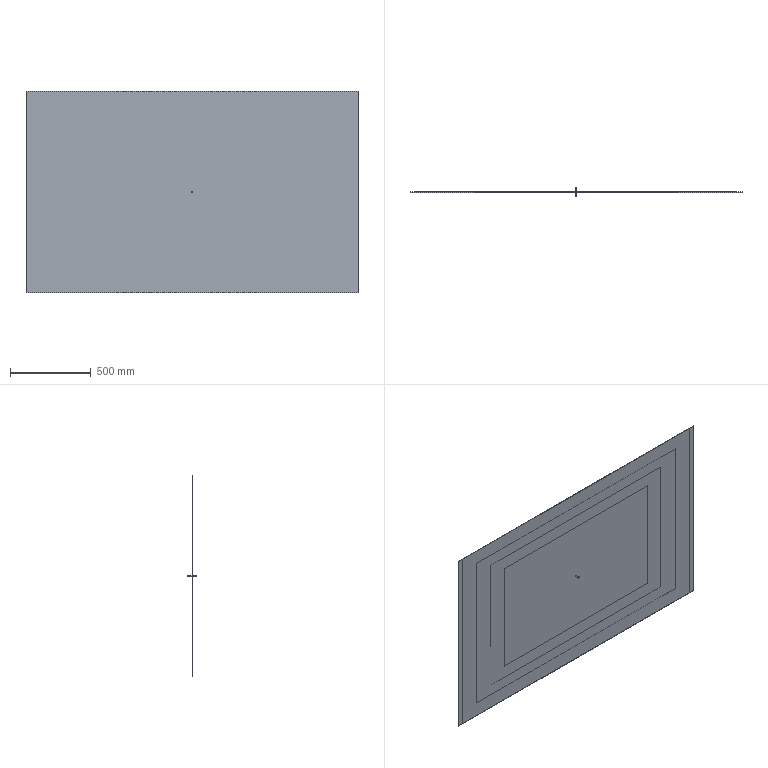Part | SolidWorks | features ICE 5, Extrusion 1 | 5 solids | 36 faces | box 2060 x 50 x 1250 mm | volume 5816564 mm3 | plane 32 | cylinder 4 | commonest cylinder face diameters 10 x4
STEP:
#1=CARTESIAN_POINT('',(1030.,-1.,625.));
#2=VERTEX_POINT('',#1);
#3=CARTESIAN_POINT('',(1030.,-1.,-625.));
#4=VERTEX_POINT('',#3);
#5=CARTESIAN_POINT('',(1030.,-1.,625.));
#6=DIRECTION('',(0.,0.,-1.));
#7=VECTOR('',#6,1000.);
#8=LINE('',#5,#7);
#9=EDGE_CURVE('',#2,#4,#8,.T.);
#10=ORIENTED_EDGE('',*,*,#9,.T.);
#11=CARTESIAN_POINT('',(1030.,1.,-625.));
#12=VERTEX_POINT('',#11);
#13=CARTESIAN_POINT('',(1030.,1.,-625.));
#14=DIRECTION('',(0.,-1.,0.));
#15=VECTOR('',#14,1000.);
#16=LINE('',#13,#15);
#17=EDGE_CURVE('',#12,#4,#16,.T.);
#18=ORIENTED_EDGE('',*,*,#17,.F.);
#19=CARTESIAN_POINT('',(1030.,1.,625.));
#20=VERTEX_POINT('',#19);
#21=CARTESIAN_POINT('',(1030.,1.,625.));
#22=DIRECTION('',(0.,0.,-1.));
#23=VECTOR('',#22,1000.);
#24=LINE('',#21,#23);
#25=EDGE_CURVE('',#20,#12,#24,.T.);
#26=ORIENTED_EDGE('',*,*,#25,.F.);
#27=CARTESIAN_POINT('',(1030.,1.,625.));
#28=DIRECTION('',(0.,-1.,0.));
#29=VECTOR('',#28,1000.);
#30=LINE('',#27,#29);
#31=EDGE_CURVE('',#20,#2,#30,.T.);
#32=ORIENTED_EDGE('',*,*,#31,.T.);
#33=EDGE_LOOP('',(#10,#18,#26,#32));
#34=FACE_OUTER_BOUND('',#33,.T.);
#35=CARTESIAN_POINT('',(1030.,1.,625.));
#36=DIRECTION('',(-1.,0.,0.));
#37=DIRECTION('',(0.,0.,1.));
#38=AXIS2_PLACEMENT_3D('',#35,#36,#37);
#39=PLANE('',#38);
#40=ADVANCED_FACE('',(#34),#39,.F.);
#41=CARTESIAN_POINT('',(-1030.,-1.,-625.));
#42=VERTEX_POINT('',#41);
#43=CARTESIAN_POINT('',(-1030.,-1.,-625.));
#44=DIRECTION('',(-1.,0.,0.));
#45=VECTOR('',#44,1000.);
#46=LINE('',#43,#45);
#47=EDGE_CURVE('',#4,#42,#46,.T.);
#48=ORIENTED_EDGE('',*,*,#47,.T.);
#49=CARTESIAN_POINT('',(-1030.,1.,-625.));
#50=VERTEX_POINT('',#49);
#51=CARTESIAN_POINT('',(-1030.,1.,-625.));
#52=DIRECTION('',(0.,-1.,0.));
#53=VECTOR('',#52,1000.);
#54=LINE('',#51,#53);
#55=EDGE_CURVE('',#50,#42,#54,.T.);
#56=ORIENTED_EDGE('',*,*,#55,.F.);
#57=CARTESIAN_POINT('',(-1030.,1.,-625.));
#58=DIRECTION('',(-1.,0.,0.));
#59=VECTOR('',#58,1000.);
#60=LINE('',#57,#59);
#61=EDGE_CURVE('',#12,#50,#60,.T.);
#62=ORIENTED_EDGE('',*,*,#61,.F.);
#63=ORIENTED_EDGE('',*,*,#17,.T.);
#64=EDGE_LOOP('',(#48,#56,#62,#63));
#65=FACE_OUTER_BOUND('',#64,.T.);
#66=CARTESIAN_POINT('',(-1030.,1.,-625.));
#67=DIRECTION('',(0.,0.,1.));
#68=DIRECTION('',(1.,0.,0.));
#69=AXIS2_PLACEMENT_3D('',#66,#67,#68);
#70=PLANE('',#69);
#71=ADVANCED_FACE('',(#65),#70,.F.);
#72=CARTESIAN_POINT('',(-1030.,-1.,625.));
#73=VERTEX_POINT('',#72);
#74=CARTESIAN_POINT('',(-1030.,-1.,625.));
#75=DIRECTION('',(0.,0.,1.));
#76=VECTOR('',#75,1000.);
#77=LINE('',#74,#76);
#78=EDGE_CURVE('',#42,#73,#77,.T.);
#79=ORIENTED_EDGE('',*,*,#78,.T.);
#80=CARTESIAN_POINT('',(-1030.,1.,625.));
#81=VERTEX_POINT('',#80);
#82=CARTESIAN_POINT('',(-1030.,1.,625.));
#83=DIRECTION('',(0.,-1.,0.));
#84=VECTOR('',#83,1000.);
#85=LINE('',#82,#84);
#86=EDGE_CURVE('',#81,#73,#85,.T.);
#87=ORIENTED_EDGE('',*,*,#86,.F.);
#88=CARTESIAN_POINT('',(-1030.,1.,625.));
#89=DIRECTION('',(0.,0.,1.));
#90=VECTOR('',#89,1000.);
#91=LINE('',#88,#90);
#92=EDGE_CURVE('',#50,#81,#91,.T.);
#93=ORIENTED_EDGE('',*,*,#92,.F.);
#94=ORIENTED_EDGE('',*,*,#55,.T.);
#95=EDGE_LOOP('',(#79,#87,#93,#94));
#96=FACE_OUTER_BOUND('',#95,.T.);
#97=CARTESIAN_POINT('',(-1030.,1.,625.));
#98=DIRECTION('',(1.,0.,0.));
#99=DIRECTION('',(0.,0.,-1.));
#100=AXIS2_PLACEMENT_3D('',#97,#98,#99);
#101=PLANE('',#100);
#102=ADVANCED_FACE('',(#96),#101,.F.);
#103=CARTESIAN_POINT('',(-1030.,-1.,625.));
#104=DIRECTION('',(1.,0.,0.));
#105=VECTOR('',#104,1000.);
#106=LINE('',#103,#105);
#107=EDGE_CURVE('',#73,#2,#106,.T.);
#108=ORIENTED_EDGE('',*,*,#107,.T.);
#109=ORIENTED_EDGE('',*,*,#31,.F.);
#110=CARTESIAN_POINT('',(-1030.,1.,625.));
#111=DIRECTION('',(1.,0.,0.));
#112=VECTOR('',#111,1000.);
#113=LINE('',#110,#112);
#114=EDGE_CURVE('',#81,#20,#113,.T.);
#115=ORIENTED_EDGE('',*,*,#114,.F.);
#116=ORIENTED_EDGE('',*,*,#86,.T.);
#117=EDGE_LOOP('',(#108,#109,#115,#116));
#118=FACE_OUTER_BOUND('',#117,.T.);
#119=CARTESIAN_POINT('',(-1030.,1.,625.));
#120=DIRECTION('',(0.,0.,-1.));
#121=DIRECTION('',(-1.,0.,0.));
#122=AXIS2_PLACEMENT_3D('',#119,#120,#121);
#123=PLANE('',#122);
#124=ADVANCED_FACE('',(#118),#123,.F.);
#125=ORIENTED_EDGE('',*,*,#25,.T.);
#126=ORIENTED_EDGE('',*,*,#61,.T.);
#127=ORIENTED_EDGE('',*,*,#92,.T.);
#128=ORIENTED_EDGE('',*,*,#114,.T.);
#129=EDGE_LOOP('',(#125,#126,#127,#128));
#130=FACE_OUTER_BOUND('',#129,.T.);
#131=CARTESIAN_POINT('',(0.,1.,0.));
#132=DIRECTION('',(0.,-1.,0.));
#133=DIRECTION('',(0.,0.,-1.));
#134=AXIS2_PLACEMENT_3D('',#131,#132,#133);
#135=PLANE('',#134);
#136=ADVANCED_FACE('',(#130),#135,.F.);
#137=ORIENTED_EDGE('',*,*,#9,.F.);
#138=ORIENTED_EDGE('',*,*,#107,.F.);
#139=ORIENTED_EDGE('',*,*,#78,.F.);
#140=ORIENTED_EDGE('',*,*,#47,.F.);
#141=EDGE_LOOP('',(#137,#138,#139,#140));
#142=FACE_OUTER_BOUND('',#141,.T.);
#143=CARTESIAN_POINT('',(0.,-1.,0.));
#144=DIRECTION('',(0.,-1.,0.));
#145=DIRECTION('',(0.,0.,-1.));
#146=AXIS2_PLACEMENT_3D('',#143,#144,#145);
#147=PLANE('',#146);
#148=ADVANCED_FACE('',(#142),#147,.T.);
#149=CLOSED_SHELL('',(#40,#71,#102,#124,#136,#148));
#150=MANIFOLD_SOLID_BREP('',#149);
#151=CARTESIAN_POINT('',(997.5,1.,625.));
#152=VERTEX_POINT('',#151);
#153=CARTESIAN_POINT('',(997.5,1.,-625.));
#154=VERTEX_POINT('',#153);
#155=CARTESIAN_POINT('',(997.5,1.,625.));
#156=DIRECTION('',(0.,0.,-1.));
#157=VECTOR('',#156,1000.);
#158=LINE('',#155,#157);
#159=EDGE_CURVE('',#152,#154,#158,.T.);
#160=ORIENTED_EDGE('',*,*,#159,.T.);
#161=CARTESIAN_POINT('',(997.5,1.1,-625.));
#162=VERTEX_POINT('',#161);
#163=CARTESIAN_POINT('',(997.5,1.1,-625.));
#164=DIRECTION('',(0.,-1.,0.));
#165=VECTOR('',#164,1000.);
#166=LINE('',#163,#165);
#167=EDGE_CURVE('',#162,#154,#166,.T.);
#168=ORIENTED_EDGE('',*,*,#167,.F.);
#169=CARTESIAN_POINT('',(997.5,1.1,625.));
#170=VERTEX_POINT('',#169);
#171=CARTESIAN_POINT('',(997.5,1.1,625.));
#172=DIRECTION('',(0.,0.,-1.));
#173=VECTOR('',#172,1000.);
#174=LINE('',#171,#173);
#175=EDGE_CURVE('',#170,#162,#174,.T.);
#176=ORIENTED_EDGE('',*,*,#175,.F.);
#177=CARTESIAN_POINT('',(997.5,1.1,625.));
#178=DIRECTION('',(0.,-1.,0.));
#179=VECTOR('',#178,1000.);
#180=LINE('',#177,#179);
#181=EDGE_CURVE('',#170,#152,#180,.T.);
#182=ORIENTED_EDGE('',*,*,#181,.T.);
#183=EDGE_LOOP('',(#160,#168,#176,#182));
#184=FACE_OUTER_BOUND('',#183,.T.);
#185=CARTESIAN_POINT('',(997.5,1.1,625.));
#186=DIRECTION('',(-1.,0.,0.));
#187=DIRECTION('',(0.,0.,1.));
#188=AXIS2_PLACEMENT_3D('',#185,#186,#187);
#189=PLANE('',#188);
#190=ADVANCED_FACE('',(#184),#189,.F.);
#191=CARTESIAN_POINT('',(-997.5,1.,-625.));
#192=VERTEX_POINT('',#191);
#193=CARTESIAN_POINT('',(-997.5,1.,-625.));
#194=DIRECTION('',(-1.,0.,0.));
#195=VECTOR('',#194,1000.);
#196=LINE('',#193,#195);
#197=EDGE_CURVE('',#154,#192,#196,.T.);
#198=ORIENTED_EDGE('',*,*,#197,.T.);
#199=CARTESIAN_POINT('',(-997.5,1.1,-625.));
#200=VERTEX_POINT('',#199);
#201=CARTESIAN_POINT('',(-997.5,1.1,-625.));
#202=DIRECTION('',(0.,-1.,0.));
#203=VECTOR('',#202,1000.);
#204=LINE('',#201,#203);
#205=EDGE_CURVE('',#200,#192,#204,.T.);
#206=ORIENTED_EDGE('',*,*,#205,.F.);
#207=CARTESIAN_POINT('',(-997.5,1.1,-625.));
#208=DIRECTION('',(-1.,0.,0.));
#209=VECTOR('',#208,1000.);
#210=LINE('',#207,#209);
#211=EDGE_CURVE('',#162,#200,#210,.T.);
#212=ORIENTED_EDGE('',*,*,#211,.F.);
#213=ORIENTED_EDGE('',*,*,#167,.T.);
#214=EDGE_LOOP('',(#198,#206,#212,#213));
#215=FACE_OUTER_BOUND('',#214,.T.);
#216=CARTESIAN_POINT('',(-997.5,1.1,-625.));
#217=DIRECTION('',(0.,0.,1.));
#218=DIRECTION('',(1.,0.,0.));
#219=AXIS2_PLACEMENT_3D('',#216,#217,#218);
#220=PLANE('',#219);
#221=ADVANCED_FACE('',(#215),#220,.F.);
#222=CARTESIAN_POINT('',(-997.5,1.,625.));
#223=VERTEX_POINT('',#222);
#224=CARTESIAN_POINT('',(-997.5,1.,625.));
#225=DIRECTION('',(0.,0.,1.));
#226=VECTOR('',#225,1000.);
#227=LINE('',#224,#226);
#228=EDGE_CURVE('',#192,#223,#227,.T.);
#229=ORIENTED_EDGE('',*,*,#228,.T.);
#230=CARTESIAN_POINT('',(-997.5,1.1,625.));
#231=VERTEX_POINT('',#230);
#232=CARTESIAN_POINT('',(-997.5,1.1,625.));
#233=DIRECTION('',(0.,-1.,0.));
#234=VECTOR('',#233,1000.);
#235=LINE('',#232,#234);
#236=EDGE_CURVE('',#231,#223,#235,.T.);
#237=ORIENTED_EDGE('',*,*,#236,.F.);
#238=CARTESIAN_POINT('',(-997.5,1.1,625.));
#239=DIRECTION('',(0.,0.,1.));
#240=VECTOR('',#239,1000.);
#241=LINE('',#238,#240);
#242=EDGE_CURVE('',#200,#231,#241,.T.);
#243=ORIENTED_EDGE('',*,*,#242,.F.);
#244=ORIENTED_EDGE('',*,*,#205,.T.);
#245=EDGE_LOOP('',(#229,#237,#243,#244));
#246=FACE_OUTER_BOUND('',#245,.T.);
#247=CARTESIAN_POINT('',(-997.5,1.1,625.));
#248=DIRECTION('',(1.,0.,0.));
#249=DIRECTION('',(0.,0.,-1.));
#250=AXIS2_PLACEMENT_3D('',#247,#248,#249);
#251=PLANE('',#250);
#252=ADVANCED_FACE('',(#246),#251,.F.);
#253=CARTESIAN_POINT('',(-997.5,1.,625.));
#254=DIRECTION('',(1.,0.,0.));
#255=VECTOR('',#254,1000.);
#256=LINE('',#253,#255);
#257=EDGE_CURVE('',#223,#152,#256,.T.);
#258=ORIENTED_EDGE('',*,*,#257,.T.);
#259=ORIENTED_EDGE('',*,*,#181,.F.);
#260=CARTESIAN_POINT('',(-997.5,1.1,625.));
#261=DIRECTION('',(1.,0.,0.));
#262=VECTOR('',#261,1000.);
#263=LINE('',#260,#262);
#264=EDGE_CURVE('',#231,#170,#263,.T.);
#265=ORIENTED_EDGE('',*,*,#264,.F.);
#266=ORIENTED_EDGE('',*,*,#236,.T.);
#267=EDGE_LOOP('',(#258,#259,#265,#266));
#268=FACE_OUTER_BOUND('',#267,.T.);
#269=CARTESIAN_POINT('',(-997.5,1.1,625.));
#270=DIRECTION('',(0.,0.,-1.));
#271=DIRECTION('',(-1.,0.,0.));
#272=AXIS2_PLACEMENT_3D('',#269,#270,#271);
#273=PLANE('',#272);
#274=ADVANCED_FACE('',(#268),#273,.F.);
#275=ORIENTED_EDGE('',*,*,#175,.T.);
#276=ORIENTED_EDGE('',*,*,#211,.T.);
#277=ORIENTED_EDGE('',*,*,#242,.T.);
#278=ORIENTED_EDGE('',*,*,#264,.T.);
#279=EDGE_LOOP('',(#275,#276,#277,#278));
#280=FACE_OUTER_BOUND('',#279,.T.);
#281=CARTESIAN_POINT('',(0.,1.1,0.));
#282=DIRECTION('',(0.,-1.,0.));
#283=DIRECTION('',(0.,0.,-1.));
#284=AXIS2_PLACEMENT_3D('',#281,#282,#283);
#285=PLANE('',#284);
#286=ADVANCED_FACE('',(#280),#285,.F.);
#287=ORIENTED_EDGE('',*,*,#159,.F.);
#288=ORIENTED_EDGE('',*,*,#257,.F.);
#289=ORIENTED_EDGE('',*,*,#228,.F.);
#290=ORIENTED_EDGE('',*,*,#197,.F.);
#291=EDGE_LOOP('',(#287,#288,#289,#290));
#292=FACE_OUTER_BOUND('',#291,.T.);
#293=CARTESIAN_POINT('',(0.,1.,0.));
#294=DIRECTION('',(0.,-1.,0.));
#295=DIRECTION('',(0.,0.,-1.));
#296=AXIS2_PLACEMENT_3D('',#293,#294,#295);
#297=PLANE('',#296);
#298=ADVANCED_FACE('',(#292),#297,.T.);
#299=CLOSED_SHELL('',(#190,#221,#252,#274,#286,#298));
#300=MANIFOLD_SOLID_BREP('',#299);
#301=CARTESIAN_POINT('',(870.,1.1,530.));
#302=VERTEX_POINT('',#301);
#303=CARTESIAN_POINT('',(870.,1.1,-530.));
#304=VERTEX_POINT('',#303);
#305=CARTESIAN_POINT('',(870.,1.1,530.));
#306=DIRECTION('',(0.,0.,-1.));
#307=VECTOR('',#306,1000.);
#308=LINE('',#305,#307);
#309=EDGE_CURVE('',#302,#304,#308,.T.);
#310=ORIENTED_EDGE('',*,*,#309,.T.);
#311=CARTESIAN_POINT('',(870.,1.2,-530.));
#312=VERTEX_POINT('',#311);
#313=CARTESIAN_POINT('',(870.,1.2,-530.));
#314=DIRECTION('',(0.,-1.,0.));
#315=VECTOR('',#314,1000.);
#316=LINE('',#313,#315);
#317=EDGE_CURVE('',#312,#304,#316,.T.);
#318=ORIENTED_EDGE('',*,*,#317,.F.);
#319=CARTESIAN_POINT('',(870.,1.2,530.));
#320=VERTEX_POINT('',#319);
#321=CARTESIAN_POINT('',(870.,1.2,530.));
#322=DIRECTION('',(0.,0.,-1.));
#323=VECTOR('',#322,1000.);
#324=LINE('',#321,#323);
#325=EDGE_CURVE('',#320,#312,#324,.T.);
#326=ORIENTED_EDGE('',*,*,#325,.F.);
#327=CARTESIAN_POINT('',(870.,1.2,530.));
#328=DIRECTION('',(0.,-1.,0.));
#329=VECTOR('',#328,1000.);
#330=LINE('',#327,#329);
#331=EDGE_CURVE('',#320,#302,#330,.T.);
#332=ORIENTED_EDGE('',*,*,#331,.T.);
#333=EDGE_LOOP('',(#310,#318,#326,#332));
#334=FACE_OUTER_BOUND('',#333,.T.);
#335=CARTESIAN_POINT('',(870.,1.2,530.));
#336=DIRECTION('',(-1.,0.,0.));
#337=DIRECTION('',(0.,0.,1.));
#338=AXIS2_PLACEMENT_3D('',#335,#336,#337);
#339=PLANE('',#338);
#340=ADVANCED_FACE('',(#334),#339,.F.);
#341=CARTESIAN_POINT('',(-870.,1.1,-530.));
#342=VERTEX_POINT('',#341);
#343=CARTESIAN_POINT('',(-870.,1.1,-530.));
#344=DIRECTION('',(-1.,0.,0.));
#345=VECTOR('',#344,1000.);
#346=LINE('',#343,#345);
#347=EDGE_CURVE('',#304,#342,#346,.T.);
#348=ORIENTED_EDGE('',*,*,#347,.T.);
#349=CARTESIAN_POINT('',(-870.,1.2,-530.));
#350=VERTEX_POINT('',#349);
#351=CARTESIAN_POINT('',(-870.,1.2,-530.));
#352=DIRECTION('',(0.,-1.,0.));
#353=VECTOR('',#352,1000.);
#354=LINE('',#351,#353);
#355=EDGE_CURVE('',#350,#342,#354,.T.);
#356=ORIENTED_EDGE('',*,*,#355,.F.);
#357=CARTESIAN_POINT('',(-870.,1.2,-530.));
#358=DIRECTION('',(-1.,0.,0.));
#359=VECTOR('',#358,1000.);
#360=LINE('',#357,#359);
#361=EDGE_CURVE('',#312,#350,#360,.T.);
#362=ORIENTED_EDGE('',*,*,#361,.F.);
#363=ORIENTED_EDGE('',*,*,#317,.T.);
#364=EDGE_LOOP('',(#348,#356,#362,#363));
#365=FACE_OUTER_BOUND('',#364,.T.);
#366=CARTESIAN_POINT('',(-870.,1.2,-530.));
#367=DIRECTION('',(0.,0.,1.));
#368=DIRECTION('',(1.,0.,0.));
#369=AXIS2_PLACEMENT_3D('',#366,#367,#368);
#370=PLANE('',#369);
#371=ADVANCED_FACE('',(#365),#370,.F.);
#372=CARTESIAN_POINT('',(-870.,1.1,530.));
#373=VERTEX_POINT('',#372);
#374=CARTESIAN_POINT('',(-870.,1.1,530.));
#375=DIRECTION('',(0.,0.,1.));
#376=VECTOR('',#375,1000.);
#377=LINE('',#374,#376);
#378=EDGE_CURVE('',#342,#373,#377,.T.);
#379=ORIENTED_EDGE('',*,*,#378,.T.);
#380=CARTESIAN_POINT('',(-870.,1.2,530.));
#381=VERTEX_POINT('',#380);
#382=CARTESIAN_POINT('',(-870.,1.2,530.));
#383=DIRECTION('',(0.,-1.,0.));
#384=VECTOR('',#383,1000.);
#385=LINE('',#382,#384);
#386=EDGE_CURVE('',#381,#373,#385,.T.);
#387=ORIENTED_EDGE('',*,*,#386,.F.);
#388=CARTESIAN_POINT('',(-870.,1.2,530.));
#389=DIRECTION('',(0.,0.,1.));
#390=VECTOR('',#389,1000.);
#391=LINE('',#388,#390);
#392=EDGE_CURVE('',#350,#381,#391,.T.);
#393=ORIENTED_EDGE('',*,*,#392,.F.);
#394=ORIENTED_EDGE('',*,*,#355,.T.);
#395=EDGE_LOOP('',(#379,#387,#393,#394));
#396=FACE_OUTER_BOUND('',#395,.T.);
#397=CARTESIAN_POINT('',(-870.,1.2,530.));
#398=DIRECTION('',(1.,0.,0.));
#399=DIRECTION('',(0.,0.,-1.));
#400=AXIS2_PLACEMENT_3D('',#397,#398,#399);
#401=PLANE('',#400);
#402=ADVANCED_FACE('',(#396),#401,.F.);
#403=CARTESIAN_POINT('',(-870.,1.1,530.));
#404=DIRECTION('',(1.,0.,0.));
#405=VECTOR('',#404,1000.);
#406=LINE('',#403,#405);
#407=EDGE_CURVE('',#373,#302,#406,.T.);
#408=ORIENTED_EDGE('',*,*,#407,.T.);
#409=ORIENTED_EDGE('',*,*,#331,.F.);
#410=CARTESIAN_POINT('',(-870.,1.2,530.));
#411=DIRECTION('',(1.,0.,0.));
#412=VECTOR('',#411,1000.);
#413=LINE('',#410,#412);
#414=EDGE_CURVE('',#381,#320,#413,.T.);
#415=ORIENTED_EDGE('',*,*,#414,.F.);
#416=ORIENTED_EDGE('',*,*,#386,.T.);
#417=EDGE_LOOP('',(#408,#409,#415,#416));
#418=FACE_OUTER_BOUND('',#417,.T.);
#419=CARTESIAN_POINT('',(-870.,1.2,530.));
#420=DIRECTION('',(0.,0.,-1.));
#421=DIRECTION('',(-1.,0.,0.));
#422=AXIS2_PLACEMENT_3D('',#419,#420,#421);
#423=PLANE('',#422);
#424=ADVANCED_FACE('',(#418),#423,.F.);
#425=ORIENTED_EDGE('',*,*,#325,.T.);
#426=ORIENTED_EDGE('',*,*,#361,.T.);
#427=ORIENTED_EDGE('',*,*,#392,.T.);
#428=ORIENTED_EDGE('',*,*,#414,.T.);
#429=EDGE_LOOP('',(#425,#426,#427,#428));
#430=FACE_OUTER_BOUND('',#429,.T.);
#431=CARTESIAN_POINT('',(0.,1.2,0.));
#432=DIRECTION('',(0.,-1.,0.));
#433=DIRECTION('',(0.,0.,-1.));
#434=AXIS2_PLACEMENT_3D('',#431,#432,#433);
#435=PLANE('',#434);
#436=ADVANCED_FACE('',(#430),#435,.F.);
#437=ORIENTED_EDGE('',*,*,#309,.F.);
#438=ORIENTED_EDGE('',*,*,#407,.F.);
#439=ORIENTED_EDGE('',*,*,#378,.F.);
#440=ORIENTED_EDGE('',*,*,#347,.F.);
#441=EDGE_LOOP('',(#437,#438,#439,#440));
#442=FACE_OUTER_BOUND('',#441,.T.);
#443=CARTESIAN_POINT('',(0.,1.1,0.));
#444=DIRECTION('',(0.,-1.,0.));
#445=DIRECTION('',(0.,0.,-1.));
#446=AXIS2_PLACEMENT_3D('',#443,#444,#445);
#447=PLANE('',#446);
#448=ADVANCED_FACE('',(#442),#447,.T.);
#449=CLOSED_SHELL('',(#340,#371,#402,#424,#436,#448));
#450=MANIFOLD_SOLID_BREP('',#449);
#451=CARTESIAN_POINT('',(745.,1.2,455.));
#452=VERTEX_POINT('',#451);
#453=CARTESIAN_POINT('',(745.,1.2,-455.));
#454=VERTEX_POINT('',#453);
#455=CARTESIAN_POINT('',(745.,1.2,455.));
#456=DIRECTION('',(0.,0.,-1.));
#457=VECTOR('',#456,1000.);
#458=LINE('',#455,#457);
#459=EDGE_CURVE('',#452,#454,#458,.T.);
#460=ORIENTED_EDGE('',*,*,#459,.T.);
#461=CARTESIAN_POINT('',(745.,1.3,-455.));
#462=VERTEX_POINT('',#461);
#463=CARTESIAN_POINT('',(745.,1.3,-455.));
#464=DIRECTION('',(0.,-1.,0.));
#465=VECTOR('',#464,1000.);
#466=LINE('',#463,#465);
#467=EDGE_CURVE('',#462,#454,#466,.T.);
#468=ORIENTED_EDGE('',*,*,#467,.F.);
#469=CARTESIAN_POINT('',(745.,1.3,455.));
#470=VERTEX_POINT('',#469);
#471=CARTESIAN_POINT('',(745.,1.3,455.));
#472=DIRECTION('',(0.,0.,-1.));
#473=VECTOR('',#472,1000.);
#474=LINE('',#471,#473);
#475=EDGE_CURVE('',#470,#462,#474,.T.);
#476=ORIENTED_EDGE('',*,*,#475,.F.);
#477=CARTESIAN_POINT('',(745.,1.3,455.));
#478=DIRECTION('',(0.,-1.,0.));
#479=VECTOR('',#478,1000.);
#480=LINE('',#477,#479);
#481=EDGE_CURVE('',#470,#452,#480,.T.);
#482=ORIENTED_EDGE('',*,*,#481,.T.);
#483=EDGE_LOOP('',(#460,#468,#476,#482));
#484=FACE_OUTER_BOUND('',#483,.T.);
#485=CARTESIAN_POINT('',(745.,1.3,455.));
#486=DIRECTION('',(-1.,0.,0.));
#487=DIRECTION('',(0.,0.,1.));
#488=AXIS2_PLACEMENT_3D('',#485,#486,#487);
#489=PLANE('',#488);
#490=ADVANCED_FACE('',(#484),#489,.F.);
#491=CARTESIAN_POINT('',(-745.,1.2,-455.));
#492=VERTEX_POINT('',#491);
#493=CARTESIAN_POINT('',(-745.,1.2,-455.));
#494=DIRECTION('',(-1.,0.,0.));
#495=VECTOR('',#494,1000.);
#496=LINE('',#493,#495);
#497=EDGE_CURVE('',#454,#492,#496,.T.);
#498=ORIENTED_EDGE('',*,*,#497,.T.);
#499=CARTESIAN_POINT('',(-745.,1.3,-455.));
#500=VERTEX_POINT('',#499);
#501=CARTESIAN_POINT('',(-745.,1.3,-455.));
#502=DIRECTION('',(0.,-1.,0.));
#503=VECTOR('',#502,1000.);
#504=LINE('',#501,#503);
#505=EDGE_CURVE('',#500,#492,#504,.T.);
#506=ORIENTED_EDGE('',*,*,#505,.F.);
#507=CARTESIAN_POINT('',(-745.,1.3,-455.));
#508=DIRECTION('',(-1.,0.,0.));
#509=VECTOR('',#508,1000.);
#510=LINE('',#507,#509);
#511=EDGE_CURVE('',#462,#500,#510,.T.);
#512=ORIENTED_EDGE('',*,*,#511,.F.);
#513=ORIENTED_EDGE('',*,*,#467,.T.);
#514=EDGE_LOOP('',(#498,#506,#512,#513));
#515=FACE_OUTER_BOUND('',#514,.T.);
#516=CARTESIAN_POINT('',(-745.,1.3,-455.));
#517=DIRECTION('',(0.,0.,1.));
#518=DIRECTION('',(1.,0.,0.));
#519=AXIS2_PLACEMENT_3D('',#516,#517,#518);
#520=PLANE('',#519);
#521=ADVANCED_FACE('',(#515),#520,.F.);
#522=CARTESIAN_POINT('',(-745.,1.2,455.));
#523=VERTEX_POINT('',#522);
#524=CARTESIAN_POINT('',(-745.,1.2,455.));
#525=DIRECTION('',(0.,0.,1.));
#526=VECTOR('',#525,1000.);
#527=LINE('',#524,#526);
#528=EDGE_CURVE('',#492,#523,#527,.T.);
#529=ORIENTED_EDGE('',*,*,#528,.T.);
#530=CARTESIAN_POINT('',(-745.,1.3,455.));
#531=VERTEX_POINT('',#530);
#532=CARTESIAN_POINT('',(-745.,1.3,455.));
#533=DIRECTION('',(0.,-1.,0.));
#534=VECTOR('',#533,1000.);
#535=LINE('',#532,#534);
#536=EDGE_CURVE('',#531,#523,#535,.T.);
#537=ORIENTED_EDGE('',*,*,#536,.F.);
#538=CARTESIAN_POINT('',(-745.,1.3,455.));
#539=DIRECTION('',(0.,0.,1.));
#540=VECTOR('',#539,1000.);
#541=LINE('',#538,#540);
#542=EDGE_CURVE('',#500,#531,#541,.T.);
#543=ORIENTED_EDGE('',*,*,#542,.F.);
#544=ORIENTED_EDGE('',*,*,#505,.T.);
#545=EDGE_LOOP('',(#529,#537,#543,#544));
#546=FACE_OUTER_BOUND('',#545,.T.);
#547=CARTESIAN_POINT('',(-745.,1.3,455.));
#548=DIRECTION('',(1.,0.,0.));
#549=DIRECTION('',(0.,0.,-1.));
#550=AXIS2_PLACEMENT_3D('',#547,#548,#549);
#551=PLANE('',#550);
#552=ADVANCED_FACE('',(#546),#551,.F.);
#553=CARTESIAN_POINT('',(-745.,1.2,455.));
#554=DIRECTION('',(1.,0.,0.));
#555=VECTOR('',#554,1000.);
#556=LINE('',#553,#555);
#557=EDGE_CURVE('',#523,#452,#556,.T.);
#558=ORIENTED_EDGE('',*,*,#557,.T.);
#559=ORIENTED_EDGE('',*,*,#481,.F.);
#560=CARTESIAN_POINT('',(-745.,1.3,455.));
#561=DIRECTION('',(1.,0.,0.));
#562=VECTOR('',#561,1000.);
#563=LINE('',#560,#562);
#564=EDGE_CURVE('',#531,#470,#563,.T.);
#565=ORIENTED_EDGE('',*,*,#564,.F.);
#566=ORIENTED_EDGE('',*,*,#536,.T.);
#567=EDGE_LOOP('',(#558,#559,#565,#566));
#568=FACE_OUTER_BOUND('',#567,.T.);
#569=CARTESIAN_POINT('',(-745.,1.3,455.));
#570=DIRECTION('',(0.,0.,-1.));
#571=DIRECTION('',(-1.,0.,0.));
#572=AXIS2_PLACEMENT_3D('',#569,#570,#571);
#573=PLANE('',#572);
#574=ADVANCED_FACE('',(#568),#573,.F.);
#575=ORIENTED_EDGE('',*,*,#475,.T.);
#576=ORIENTED_EDGE('',*,*,#511,.T.);
#577=ORIENTED_EDGE('',*,*,#542,.T.);
#578=ORIENTED_EDGE('',*,*,#564,.T.);
#579=EDGE_LOOP('',(#575,#576,#577,#578));
#580=FACE_OUTER_BOUND('',#579,.T.);
#581=CARTESIAN_POINT('',(0.,1.3,0.));
#582=DIRECTION('',(0.,-1.,0.));
#583=DIRECTION('',(0.,0.,-1.));
#584=AXIS2_PLACEMENT_3D('',#581,#582,#583);
#585=PLANE('',#584);
#586=ADVANCED_FACE('',(#580),#585,.F.);
#587=ORIENTED_EDGE('',*,*,#459,.F.);
#588=ORIENTED_EDGE('',*,*,#557,.F.);
#589=ORIENTED_EDGE('',*,*,#528,.F.);
#590=ORIENTED_EDGE('',*,*,#497,.F.);
#591=EDGE_LOOP('',(#587,#588,#589,#590));
#592=FACE_OUTER_BOUND('',#591,.T.);
#593=CARTESIAN_POINT('',(0.,1.2,0.));
#594=DIRECTION('',(0.,-1.,0.));
#595=DIRECTION('',(0.,0.,-1.));
#596=AXIS2_PLACEMENT_3D('',#593,#594,#595);
#597=PLANE('',#596);
#598=ADVANCED_FACE('',(#592),#597,.T.);
#599=CLOSED_SHELL('',(#490,#521,#552,#574,#586,#598));
#600=MANIFOLD_SOLID_BREP('',#599);
#601=CARTESIAN_POINT('',(0.,26.4,5.));
#602=VERTEX_POINT('',#601);
#603=CARTESIAN_POINT('',(0.,26.4,-5.));
#604=VERTEX_POINT('',#603);
#605=CARTESIAN_POINT('',(0.,26.4,0.));
#606=DIRECTION('',(0.,1.,0.));
#607=DIRECTION('',(0.,0.,1.));
#608=AXIS2_PLACEMENT_3D('',#605,#606,#607);
#609=CIRCLE('',#608,5.);
#610=EDGE_CURVE('',#602,#604,#609,.T.);
#611=ORIENTED_EDGE('',*,*,#610,.F.);
#612=CARTESIAN_POINT('',(0.,1.4,5.));
#613=VERTEX_POINT('',#612);
#614=CARTESIAN_POINT('',(0.,26.4,5.));
#615=DIRECTION('',(0.,-1.,0.));
#616=VECTOR('',#615,1000.);
#617=LINE('',#614,#616);
#618=EDGE_CURVE('',#602,#613,#617,.T.);
#619=ORIENTED_EDGE('',*,*,#618,.T.);
#620=CARTESIAN_POINT('',(0.,1.4,-5.));
#621=VERTEX_POINT('',#620);
#622=CARTESIAN_POINT('',(0.,1.4,0.));
#623=DIRECTION('',(0.,1.,0.));
#624=DIRECTION('',(0.,0.,-1.));
#625=AXIS2_PLACEMENT_3D('',#622,#623,#624);
#626=CIRCLE('',#625,5.);
#627=EDGE_CURVE('',#613,#621,#626,.T.);
#628=ORIENTED_EDGE('',*,*,#627,.T.);
#629=CARTESIAN_POINT('',(0.,26.4,-5.));
#630=DIRECTION('',(0.,-1.,0.));
#631=VECTOR('',#630,1000.);
#632=LINE('',#629,#631);
#633=EDGE_CURVE('',#604,#621,#632,.T.);
#634=ORIENTED_EDGE('',*,*,#633,.F.);
#635=EDGE_LOOP('',(#611,#619,#628,#634));
#636=FACE_OUTER_BOUND('',#635,.T.);
#637=CARTESIAN_POINT('',(0.,26.4,0.));
#638=DIRECTION('',(0.,-1.,0.));
#639=DIRECTION('',(0.,0.,-1.));
#640=AXIS2_PLACEMENT_3D('',#637,#638,#639);
#641=CYLINDRICAL_SURFACE('',#640,5.);
#642=ADVANCED_FACE('',(#636),#641,.T.);
#643=CARTESIAN_POINT('',(0.,1.3,5.));
#644=VERTEX_POINT('',#643);
#645=CARTESIAN_POINT('',(0.,1.3,-5.));
#646=VERTEX_POINT('',#645);
#647=CARTESIAN_POINT('',(0.,1.3,0.));
#648=DIRECTION('',(0.,1.,0.));
#649=DIRECTION('',(0.,0.,-1.));
#650=AXIS2_PLACEMENT_3D('',#647,#648,#649);
#651=CIRCLE('',#650,5.);
#652=EDGE_CURVE('',#644,#646,#651,.T.);
#653=ORIENTED_EDGE('',*,*,#652,.F.);
#654=CARTESIAN_POINT('',(0.,-23.6,5.));
#655=VERTEX_POINT('',#654);
#656=CARTESIAN_POINT('',(0.,26.4,5.));
#657=DIRECTION('',(0.,-1.,0.));
#658=VECTOR('',#657,1000.);
#659=LINE('',#656,#658);
#660=EDGE_CURVE('',#644,#655,#659,.T.);
#661=ORIENTED_EDGE('',*,*,#660,.T.);
#662=CARTESIAN_POINT('',(0.,-23.6,-5.));
#663=VERTEX_POINT('',#662);
#664=CARTESIAN_POINT('',(0.,-23.6,0.));
#665=DIRECTION('',(0.,1.,0.));
#666=DIRECTION('',(0.,0.,1.));
#667=AXIS2_PLACEMENT_3D('',#664,#665,#666);
#668=CIRCLE('',#667,5.);
#669=EDGE_CURVE('',#655,#663,#668,.T.);
#670=ORIENTED_EDGE('',*,*,#669,.T.);
#671=CARTESIAN_POINT('',(0.,26.4,-5.));
#672=DIRECTION('',(0.,-1.,0.));
#673=VECTOR('',#672,1000.);
#674=LINE('',#671,#673);
#675=EDGE_CURVE('',#646,#663,#674,.T.);
#676=ORIENTED_EDGE('',*,*,#675,.F.);
#677=EDGE_LOOP('',(#653,#661,#670,#676));
#678=FACE_OUTER_BOUND('',#677,.T.);
#679=CARTESIAN_POINT('',(0.,26.4,0.));
#680=DIRECTION('',(0.,-1.,0.));
#681=DIRECTION('',(0.,0.,-1.));
#682=AXIS2_PLACEMENT_3D('',#679,#680,#681);
#683=CYLINDRICAL_SURFACE('',#682,5.);
#684=ADVANCED_FACE('',(#678),#683,.T.);
#685=CARTESIAN_POINT('',(630.,1.4,370.));
#686=VERTEX_POINT('',#685);
#687=CARTESIAN_POINT('',(630.,1.4,-370.));
#688=VERTEX_POINT('',#687);
#689=CARTESIAN_POINT('',(630.,1.4,370.));
#690=DIRECTION('',(0.,0.,-1.));
#691=VECTOR('',#690,1000.);
#692=LINE('',#689,#691);
#693=EDGE_CURVE('',#686,#688,#692,.T.);
#694=ORIENTED_EDGE('',*,*,#693,.T.);
#695=CARTESIAN_POINT('',(-630.,1.4,-370.));
#696=VERTEX_POINT('',#695);
#697=CARTESIAN_POINT('',(-630.,1.4,-370.));
#698=DIRECTION('',(-1.,0.,0.));
#699=VECTOR('',#698,1000.);
#700=LINE('',#697,#699);
#701=EDGE_CURVE('',#688,#696,#700,.T.);
#702=ORIENTED_EDGE('',*,*,#701,.T.);
#703=CARTESIAN_POINT('',(-630.,1.4,370.));
#704=VERTEX_POINT('',#703);
#705=CARTESIAN_POINT('',(-630.,1.4,370.));
#706=DIRECTION('',(0.,0.,1.));
#707=VECTOR('',#706,1000.);
#708=LINE('',#705,#707);
#709=EDGE_CURVE('',#696,#704,#708,.T.);
#710=ORIENTED_EDGE('',*,*,#709,.T.);
#711=CARTESIAN_POINT('',(-630.,1.4,370.));
#712=DIRECTION('',(1.,0.,0.));
#713=VECTOR('',#712,1000.);
#714=LINE('',#711,#713);
#715=EDGE_CURVE('',#704,#686,#714,.T.);
#716=ORIENTED_EDGE('',*,*,#715,.T.);
#717=EDGE_LOOP('',(#694,#702,#710,#716));
#718=FACE_OUTER_BOUND('',#717,.T.);
#719=CARTESIAN_POINT('',(0.,1.4,0.));
#720=DIRECTION('',(0.,1.,0.));
#721=DIRECTION('',(0.,0.,-1.));
#722=AXIS2_PLACEMENT_3D('',#719,#720,#721);
#723=CIRCLE('',#722,5.);
#724=EDGE_CURVE('',#621,#613,#723,.T.);
#725=ORIENTED_EDGE('',*,*,#724,.F.);
#726=ORIENTED_EDGE('',*,*,#627,.F.);
#727=EDGE_LOOP('',(#725,#726));
#728=FACE_BOUND('',#727,.T.);
#729=CARTESIAN_POINT('',(0.,1.4,0.));
#730=DIRECTION('',(0.,-1.,0.));
#731=DIRECTION('',(0.,0.,-1.));
#732=AXIS2_PLACEMENT_3D('',#729,#730,#731);
#733=PLANE('',#732);
#734=ADVANCED_FACE('',(#718,#728),#733,.F.);
#735=CARTESIAN_POINT('',(630.,1.3,370.));
#736=VERTEX_POINT('',#735);
#737=CARTESIAN_POINT('',(630.,1.3,-370.));
#738=VERTEX_POINT('',#737);
#739=CARTESIAN_POINT('',(630.,1.3,370.));
#740=DIRECTION('',(0.,0.,-1.));
#741=VECTOR('',#740,1000.);
#742=LINE('',#739,#741);
#743=EDGE_CURVE('',#736,#738,#742,.T.);
#744=ORIENTED_EDGE('',*,*,#743,.F.);
#745=CARTESIAN_POINT('',(-630.,1.3,370.));
#746=VERTEX_POINT('',#745);
#747=CARTESIAN_POINT('',(-630.,1.3,370.));
#748=DIRECTION('',(1.,0.,0.));
#749=VECTOR('',#748,1000.);
#750=LINE('',#747,#749);
#751=EDGE_CURVE('',#746,#736,#750,.T.);
#752=ORIENTED_EDGE('',*,*,#751,.F.);
#753=CARTESIAN_POINT('',(-630.,1.3,-370.));
#754=VERTEX_POINT('',#753);
#755=CARTESIAN_POINT('',(-630.,1.3,370.));
#756=DIRECTION('',(0.,0.,1.));
#757=VECTOR('',#756,1000.);
#758=LINE('',#755,#757);
#759=EDGE_CURVE('',#754,#746,#758,.T.);
#760=ORIENTED_EDGE('',*,*,#759,.F.);
#761=CARTESIAN_POINT('',(-630.,1.3,-370.));
#762=DIRECTION('',(-1.,0.,0.));
#763=VECTOR('',#762,1000.);
#764=LINE('',#761,#763);
#765=EDGE_CURVE('',#738,#754,#764,.T.);
#766=ORIENTED_EDGE('',*,*,#765,.F.);
#767=EDGE_LOOP('',(#744,#752,#760,#766));
#768=FACE_OUTER_BOUND('',#767,.T.);
#769=CARTESIAN_POINT('',(0.,1.3,0.));
#770=DIRECTION('',(0.,1.,0.));
#771=DIRECTION('',(0.,0.,-1.));
#772=AXIS2_PLACEMENT_3D('',#769,#770,#771);
#773=CIRCLE('',#772,5.);
#774=EDGE_CURVE('',#646,#644,#773,.T.);
#775=ORIENTED_EDGE('',*,*,#774,.T.);
#776=ORIENTED_EDGE('',*,*,#652,.T.);
#777=EDGE_LOOP('',(#775,#776));
#778=FACE_BOUND('',#777,.T.);
#779=CARTESIAN_POINT('',(0.,1.3,0.));
#780=DIRECTION('',(0.,-1.,0.));
#781=DIRECTION('',(0.,0.,-1.));
#782=AXIS2_PLACEMENT_3D('',#779,#780,#781);
#783=PLANE('',#782);
#784=ADVANCED_FACE('',(#768,#778),#783,.T.);
#785=ORIENTED_EDGE('',*,*,#743,.T.);
#786=CARTESIAN_POINT('',(630.,1.4,-370.));
#787=DIRECTION('',(0.,-1.,0.));
#788=VECTOR('',#787,1000.);
#789=LINE('',#786,#788);
#790=EDGE_CURVE('',#688,#738,#789,.T.);
#791=ORIENTED_EDGE('',*,*,#790,.F.);
#792=ORIENTED_EDGE('',*,*,#693,.F.);
#793=CARTESIAN_POINT('',(630.,1.4,370.));
#794=DIRECTION('',(0.,-1.,0.));
#795=VECTOR('',#794,1000.);
#796=LINE('',#793,#795);
#797=EDGE_CURVE('',#686,#736,#796,.T.);
#798=ORIENTED_EDGE('',*,*,#797,.T.);
#799=EDGE_LOOP('',(#785,#791,#792,#798));
#800=FACE_OUTER_BOUND('',#799,.T.);
#801=CARTESIAN_POINT('',(630.,1.4,370.));
#802=DIRECTION('',(-1.,0.,0.));
#803=DIRECTION('',(0.,0.,1.));
#804=AXIS2_PLACEMENT_3D('',#801,#802,#803);
#805=PLANE('',#804);
#806=ADVANCED_FACE('',(#800),#805,.F.);
#807=ORIENTED_EDGE('',*,*,#765,.T.);
#808=CARTESIAN_POINT('',(-630.,1.4,-370.));
#809=DIRECTION('',(0.,-1.,0.));
#810=VECTOR('',#809,1000.);
#811=LINE('',#808,#810);
#812=EDGE_CURVE('',#696,#754,#811,.T.);
#813=ORIENTED_EDGE('',*,*,#812,.F.);
#814=ORIENTED_EDGE('',*,*,#701,.F.);
#815=ORIENTED_EDGE('',*,*,#790,.T.);
#816=EDGE_LOOP('',(#807,#813,#814,#815));
#817=FACE_OUTER_BOUND('',#816,.T.);
#818=CARTESIAN_POINT('',(-630.,1.4,-370.));
#819=DIRECTION('',(0.,0.,1.));
#820=DIRECTION('',(1.,0.,0.));
#821=AXIS2_PLACEMENT_3D('',#818,#819,#820);
#822=PLANE('',#821);
#823=ADVANCED_FACE('',(#817),#822,.F.);
#824=ORIENTED_EDGE('',*,*,#759,.T.);
#825=CARTESIAN_POINT('',(-630.,1.4,370.));
#826=DIRECTION('',(0.,-1.,0.));
#827=VECTOR('',#826,1000.);
#828=LINE('',#825,#827);
#829=EDGE_CURVE('',#704,#746,#828,.T.);
#830=ORIENTED_EDGE('',*,*,#829,.F.);
#831=ORIENTED_EDGE('',*,*,#709,.F.);
#832=ORIENTED_EDGE('',*,*,#812,.T.);
#833=EDGE_LOOP('',(#824,#830,#831,#832));
#834=FACE_OUTER_BOUND('',#833,.T.);
#835=CARTESIAN_POINT('',(-630.,1.4,370.));
#836=DIRECTION('',(1.,0.,0.));
#837=DIRECTION('',(0.,0.,-1.));
#838=AXIS2_PLACEMENT_3D('',#835,#836,#837);
#839=PLANE('',#838);
#840=ADVANCED_FACE('',(#834),#839,.F.);
#841=ORIENTED_EDGE('',*,*,#751,.T.);
#842=ORIENTED_EDGE('',*,*,#797,.F.);
#843=ORIENTED_EDGE('',*,*,#715,.F.);
#844=ORIENTED_EDGE('',*,*,#829,.T.);
#845=EDGE_LOOP('',(#841,#842,#843,#844));
#846=FACE_OUTER_BOUND('',#845,.T.);
#847=CARTESIAN_POINT('',(-630.,1.4,370.));
#848=DIRECTION('',(0.,0.,-1.));
#849=DIRECTION('',(-1.,0.,0.));
#850=AXIS2_PLACEMENT_3D('',#847,#848,#849);
#851=PLANE('',#850);
#852=ADVANCED_FACE('',(#846),#851,.F.);
#853=CARTESIAN_POINT('',(0.,-23.6,0.));
#854=DIRECTION('',(0.,1.,0.));
#855=DIRECTION('',(0.,0.,1.));
#856=AXIS2_PLACEMENT_3D('',#853,#854,#855);
#857=CIRCLE('',#856,5.);
#858=EDGE_CURVE('',#663,#655,#857,.T.);
#859=ORIENTED_EDGE('',*,*,#858,.F.);
#860=ORIENTED_EDGE('',*,*,#669,.F.);
#861=EDGE_LOOP('',(#859,#860));
#862=FACE_OUTER_BOUND('',#861,.T.);
#863=CARTESIAN_POINT('',(0.,-23.6,0.));
#864=DIRECTION('',(0.,1.,0.));
#865=DIRECTION('',(0.,0.,1.));
#866=AXIS2_PLACEMENT_3D('',#863,#864,#865);
#867=PLANE('',#866);
#868=ADVANCED_FACE('',(#862),#867,.F.);
#869=ORIENTED_EDGE('',*,*,#660,.F.);
#870=ORIENTED_EDGE('',*,*,#774,.F.);
#871=ORIENTED_EDGE('',*,*,#675,.T.);
#872=ORIENTED_EDGE('',*,*,#858,.T.);
#873=EDGE_LOOP('',(#869,#870,#871,#872));
#874=FACE_OUTER_BOUND('',#873,.T.);
#875=CARTESIAN_POINT('',(0.,26.4,0.));
#876=DIRECTION('',(0.,-1.,0.));
#877=DIRECTION('',(0.,0.,-1.));
#878=AXIS2_PLACEMENT_3D('',#875,#876,#877);
#879=CYLINDRICAL_SURFACE('',#878,5.);
#880=ADVANCED_FACE('',(#874),#879,.T.);
#881=ORIENTED_EDGE('',*,*,#618,.F.);
#882=CARTESIAN_POINT('',(0.,26.4,0.));
#883=DIRECTION('',(0.,1.,0.));
#884=DIRECTION('',(0.,0.,1.));
#885=AXIS2_PLACEMENT_3D('',#882,#883,#884);
#886=CIRCLE('',#885,5.);
#887=EDGE_CURVE('',#604,#602,#886,.T.);
#888=ORIENTED_EDGE('',*,*,#887,.F.);
#889=ORIENTED_EDGE('',*,*,#633,.T.);
#890=ORIENTED_EDGE('',*,*,#724,.T.);
#891=EDGE_LOOP('',(#881,#888,#889,#890));
#892=FACE_OUTER_BOUND('',#891,.T.);
#893=CARTESIAN_POINT('',(0.,26.4,0.));
#894=DIRECTION('',(0.,-1.,0.));
#895=DIRECTION('',(0.,0.,-1.));
#896=AXIS2_PLACEMENT_3D('',#893,#894,#895);
#897=CYLINDRICAL_SURFACE('',#896,5.);
#898=ADVANCED_FACE('',(#892),#897,.T.);
#899=ORIENTED_EDGE('',*,*,#887,.T.);
#900=ORIENTED_EDGE('',*,*,#610,.T.);
#901=EDGE_LOOP('',(#899,#900));
#902=FACE_OUTER_BOUND('',#901,.T.);
#903=CARTESIAN_POINT('',(0.,26.4,0.));
#904=DIRECTION('',(0.,1.,0.));
#905=DIRECTION('',(0.,0.,1.));
#906=AXIS2_PLACEMENT_3D('',#903,#904,#905);
#907=PLANE('',#906);
#908=ADVANCED_FACE('',(#902),#907,.T.);
#909=CLOSED_SHELL('',(#642,#684,#734,#784,#806,#823,#840,#852,#868,#880,#898,#908));
#910=MANIFOLD_SOLID_BREP('',#909);
#911=CARTESIAN_POINT('',(0.,0.,0.));
#912=DIRECTION('',(0.,0.,1.));
#913=DIRECTION('',(1.,0.,0.));
#914=AXIS2_PLACEMENT_3D('',#911,#912,#913);
#915=(LENGTH_UNIT()NAMED_UNIT(*)SI_UNIT(.MILLI.,.METRE.));
#916=UNCERTAINTY_MEASURE_WITH_UNIT(LENGTH_MEASURE(0.00001),#915,'','');
#917=(NAMED_UNIT(*)PLANE_ANGLE_UNIT()SI_UNIT($,.RADIAN.));
#918=(NAMED_UNIT(*)SI_UNIT($,.STERADIAN.)SOLID_ANGLE_UNIT());
#919=(GEOMETRIC_REPRESENTATION_CONTEXT(3)GLOBAL_UNCERTAINTY_ASSIGNED_CONTEXT((#916))GLOBAL_UNIT_ASSIGNED_CONTEXT((#915,#917,#918))REPRESENTATION_CONTEXT('',''));
#920=ADVANCED_BREP_SHAPE_REPRESENTATION('',(#150,#300,#450,#600,#910,#914),#919);